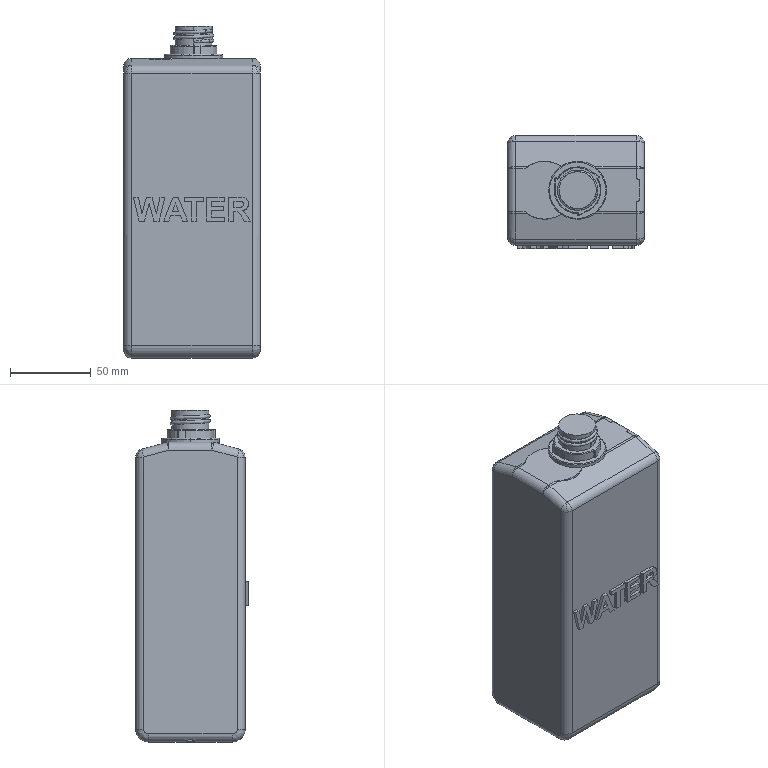Part | SolidWorks | features BaseBody 2 | 2 solids | 185 faces | box 85 x 70 x 206 mm | volume 1070549 mm3 | plane 86 | cylinder 45 | spline 24 | sphere 22 | torus 8 | commonest cylinder face diameters 10 x18 1 x6 23 x5 36 x4 20 x3 29 x3